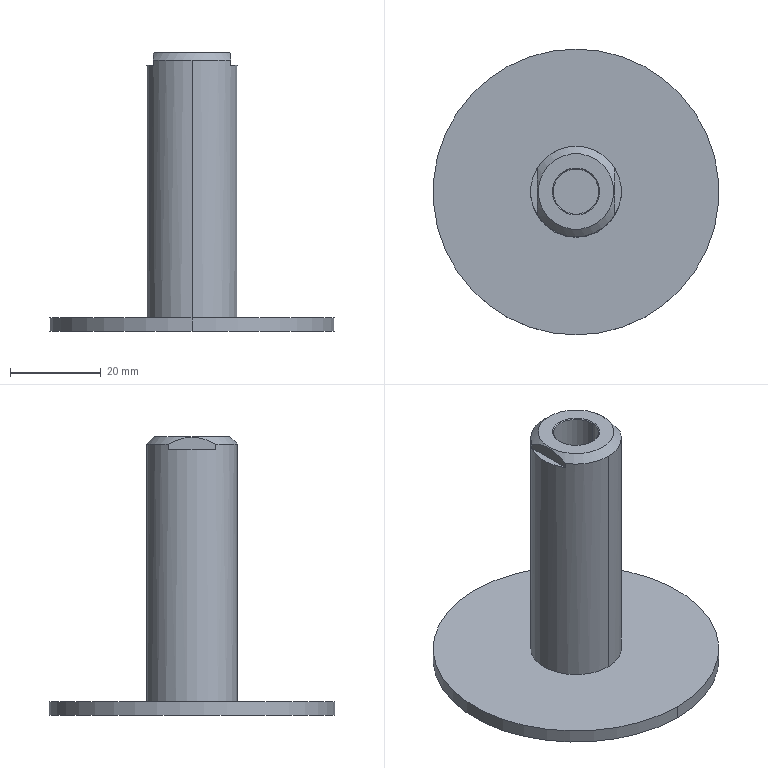Part | SolidWorks | features BaseBody 1 | 1 solid | 18 faces | box 63 x 63 x 61.5 mm | volume 26825 mm3 | plane 8 | cylinder 6 | cone 4 | commonest cylinder face diameters 10 x2 20 x2 63 x2
STEP:
#1=CARTESIAN_POINT('',(0.,-31.5,-49.667));
#2=VERTEX_POINT('',#1);
#3=CARTESIAN_POINT('',(0.,31.5,-49.667));
#4=VERTEX_POINT('',#3);
#5=CARTESIAN_POINT('',(0.,0.,-49.667));
#6=DIRECTION('',(0.,0.,1.));
#7=DIRECTION('',(0.,-1.,0.));
#8=AXIS2_PLACEMENT_3D('',#5,#6,#7);
#9=CIRCLE('',#8,31.5);
#10=EDGE_CURVE('',#2,#4,#9,.T.);
#11=ORIENTED_EDGE('',*,*,#10,.T.);
#12=CARTESIAN_POINT('',(0.,31.5,-46.667));
#13=VERTEX_POINT('',#12);
#14=CARTESIAN_POINT('',(0.,31.5,2.833));
#15=DIRECTION('',(0.,0.,1.));
#16=VECTOR('',#15,1000.);
#17=LINE('',#14,#16);
#18=EDGE_CURVE('',#4,#13,#17,.T.);
#19=ORIENTED_EDGE('',*,*,#18,.T.);
#20=CARTESIAN_POINT('',(0.,-31.5,-46.667));
#21=VERTEX_POINT('',#20);
#22=CARTESIAN_POINT('',(0.,0.,-46.667));
#23=DIRECTION('',(0.,0.,-1.));
#24=DIRECTION('',(0.,-1.,0.));
#25=AXIS2_PLACEMENT_3D('',#22,#23,#24);
#26=CIRCLE('',#25,31.5);
#27=EDGE_CURVE('',#13,#21,#26,.T.);
#28=ORIENTED_EDGE('',*,*,#27,.T.);
#29=CARTESIAN_POINT('',(0.,-31.5,2.833));
#30=DIRECTION('',(0.,0.,1.));
#31=VECTOR('',#30,1000.);
#32=LINE('',#29,#31);
#33=EDGE_CURVE('',#2,#21,#32,.T.);
#34=ORIENTED_EDGE('',*,*,#33,.F.);
#35=EDGE_LOOP('',(#11,#19,#28,#34));
#36=FACE_OUTER_BOUND('',#35,.T.);
#37=CARTESIAN_POINT('',(0.,0.,2.833));
#38=DIRECTION('',(0.,0.,1.));
#39=DIRECTION('',(0.,-1.,0.));
#40=AXIS2_PLACEMENT_3D('',#37,#38,#39);
#41=CYLINDRICAL_SURFACE('',#40,31.5);
#42=ADVANCED_FACE('',(#36),#41,.T.);
#43=CARTESIAN_POINT('',(0.,-10.,-46.667));
#44=VERTEX_POINT('',#43);
#45=CARTESIAN_POINT('',(0.,10.,-46.667));
#46=VERTEX_POINT('',#45);
#47=CARTESIAN_POINT('',(0.,0.,-46.667));
#48=DIRECTION('',(0.,0.,1.));
#49=DIRECTION('',(0.,-1.,0.));
#50=AXIS2_PLACEMENT_3D('',#47,#48,#49);
#51=CIRCLE('',#50,10.);
#52=EDGE_CURVE('',#44,#46,#51,.T.);
#53=ORIENTED_EDGE('',*,*,#52,.T.);
#54=CARTESIAN_POINT('',(0.,10.,10.167));
#55=VERTEX_POINT('',#54);
#56=CARTESIAN_POINT('',(0.,10.,2.833));
#57=DIRECTION('',(0.,0.,1.));
#58=VECTOR('',#57,1000.);
#59=LINE('',#56,#58);
#60=EDGE_CURVE('',#46,#55,#59,.T.);
#61=ORIENTED_EDGE('',*,*,#60,.T.);
#62=CARTESIAN_POINT('',(8.5,5.268,10.167));
#63=VERTEX_POINT('',#62);
#64=CARTESIAN_POINT('',(0.,0.,10.167));
#65=DIRECTION('',(0.,0.,-1.));
#66=DIRECTION('',(0.,-1.,0.));
#67=AXIS2_PLACEMENT_3D('',#64,#65,#66);
#68=CIRCLE('',#67,10.);
#69=EDGE_CURVE('',#55,#63,#68,.T.);
#70=ORIENTED_EDGE('',*,*,#69,.T.);
#71=CARTESIAN_POINT('',(8.5,5.268,9.033));
#72=VERTEX_POINT('',#71);
#73=CARTESIAN_POINT('',(8.5,5.268,9.033));
#74=DIRECTION('',(0.,0.,-1.));
#75=VECTOR('',#74,1000.);
#76=LINE('',#73,#75);
#77=EDGE_CURVE('',#63,#72,#76,.T.);
#78=ORIENTED_EDGE('',*,*,#77,.T.);
#79=CARTESIAN_POINT('',(8.5,-5.268,9.033));
#80=VERTEX_POINT('',#79);
#81=CARTESIAN_POINT('',(0.,0.,9.033));
#82=DIRECTION('',(0.,0.,-1.));
#83=DIRECTION('',(0.,-1.,0.));
#84=AXIS2_PLACEMENT_3D('',#81,#82,#83);
#85=CIRCLE('',#84,10.);
#86=EDGE_CURVE('',#72,#80,#85,.T.);
#87=ORIENTED_EDGE('',*,*,#86,.T.);
#88=CARTESIAN_POINT('',(8.5,-5.268,10.167));
#89=VERTEX_POINT('',#88);
#90=CARTESIAN_POINT('',(8.5,-5.268,9.033));
#91=DIRECTION('',(0.,0.,1.));
#92=VECTOR('',#91,1000.);
#93=LINE('',#90,#92);
#94=EDGE_CURVE('',#80,#89,#93,.T.);
#95=ORIENTED_EDGE('',*,*,#94,.T.);
#96=CARTESIAN_POINT('',(0.,-10.,10.167));
#97=VERTEX_POINT('',#96);
#98=CARTESIAN_POINT('',(0.,0.,10.167));
#99=DIRECTION('',(0.,0.,-1.));
#100=DIRECTION('',(0.,-1.,0.));
#101=AXIS2_PLACEMENT_3D('',#98,#99,#100);
#102=CIRCLE('',#101,10.);
#103=EDGE_CURVE('',#89,#97,#102,.T.);
#104=ORIENTED_EDGE('',*,*,#103,.T.);
#105=CARTESIAN_POINT('',(0.,-10.,2.833));
#106=DIRECTION('',(0.,0.,1.));
#107=VECTOR('',#106,1000.);
#108=LINE('',#105,#107);
#109=EDGE_CURVE('',#44,#97,#108,.T.);
#110=ORIENTED_EDGE('',*,*,#109,.F.);
#111=EDGE_LOOP('',(#53,#61,#70,#78,#87,#95,#104,#110));
#112=FACE_OUTER_BOUND('',#111,.T.);
#113=CARTESIAN_POINT('',(0.,0.,2.833));
#114=DIRECTION('',(0.,0.,1.));
#115=DIRECTION('',(0.,-1.,0.));
#116=AXIS2_PLACEMENT_3D('',#113,#114,#115);
#117=CYLINDRICAL_SURFACE('',#116,10.);
#118=ADVANCED_FACE('',(#112),#117,.T.);
#119=CARTESIAN_POINT('',(-8.333,0.,11.833));
#120=VERTEX_POINT('',#119);
#121=CARTESIAN_POINT('',(8.333,0.,11.833));
#122=VERTEX_POINT('',#121);
#123=CARTESIAN_POINT('',(0.,0.,11.833));
#124=DIRECTION('',(0.,0.,-1.));
#125=DIRECTION('',(-1.,0.,0.));
#126=AXIS2_PLACEMENT_3D('',#123,#124,#125);
#127=CIRCLE('',#126,8.333);
#128=EDGE_CURVE('',#120,#122,#127,.T.);
#129=ORIENTED_EDGE('',*,*,#128,.T.);
#130=CARTESIAN_POINT('',(8.5,0.,11.667));
#131=VERTEX_POINT('',#130);
#132=CARTESIAN_POINT('',(10.,0.,10.167));
#133=DIRECTION('',(0.7071,0.,-0.7071));
#134=VECTOR('',#133,1000.);
#135=LINE('',#132,#134);
#136=EDGE_CURVE('',#122,#131,#135,.T.);
#137=ORIENTED_EDGE('',*,*,#136,.T.);
#138=CARTESIAN_POINT('',(8.5,0.,11.667));
#139=CARTESIAN_POINT('',(8.5,0.459,11.667));
#140=CARTESIAN_POINT('',(8.5,0.9179,11.629));
#141=CARTESIAN_POINT('',(8.5,1.835,11.483));
#142=CARTESIAN_POINT('',(8.5,2.287,11.374));
#143=CARTESIAN_POINT('',(8.5,3.607,10.971));
#144=CARTESIAN_POINT('',(8.5,4.448,10.599));
#145=CARTESIAN_POINT('',(8.5,5.268,10.167));
#146=B_SPLINE_CURVE_WITH_KNOTS('',3,(#138,#139,#140,#141,#142,#143,#144,#145),.UNSPECIFIED.,.F.,.F.,(4,2,2,4),(0.005508,0.006884,0.008261,0.01101),.UNSPECIFIED.);
#147=EDGE_CURVE('',#131,#63,#146,.T.);
#148=ORIENTED_EDGE('',*,*,#147,.T.);
#149=ORIENTED_EDGE('',*,*,#69,.F.);
#150=CARTESIAN_POINT('',(-8.5,5.268,10.167));
#151=VERTEX_POINT('',#150);
#152=CARTESIAN_POINT('',(0.,0.,10.167));
#153=DIRECTION('',(0.,0.,-1.));
#154=DIRECTION('',(0.,-1.,0.));
#155=AXIS2_PLACEMENT_3D('',#152,#153,#154);
#156=CIRCLE('',#155,10.);
#157=EDGE_CURVE('',#151,#55,#156,.T.);
#158=ORIENTED_EDGE('',*,*,#157,.F.);
#159=CARTESIAN_POINT('',(-8.5,0.,11.667));
#160=VERTEX_POINT('',#159);
#161=CARTESIAN_POINT('',(-8.5,5.268,10.167));
#162=CARTESIAN_POINT('',(-8.5,4.448,10.599));
#163=CARTESIAN_POINT('',(-8.5,3.607,10.971));
#164=CARTESIAN_POINT('',(-8.5,2.288,11.374));
#165=CARTESIAN_POINT('',(-8.5,1.837,11.482));
#166=CARTESIAN_POINT('',(-8.5,0.9184,11.629));
#167=CARTESIAN_POINT('',(-8.5,0.4592,11.667));
#168=CARTESIAN_POINT('',(-8.5,0.,11.667));
#169=B_SPLINE_CURVE_WITH_KNOTS('',3,(#161,#162,#163,#164,#165,#166,#167,#168),.UNSPECIFIED.,.F.,.F.,(4,2,2,4),(0.,0.002754,0.004131,0.005508),.UNSPECIFIED.);
#170=EDGE_CURVE('',#151,#160,#169,.T.);
#171=ORIENTED_EDGE('',*,*,#170,.T.);
#172=CARTESIAN_POINT('',(-10.,0.,10.167));
#173=DIRECTION('',(-0.7071,0.,-0.7071));
#174=VECTOR('',#173,1000.);
#175=LINE('',#172,#174);
#176=EDGE_CURVE('',#120,#160,#175,.T.);
#177=ORIENTED_EDGE('',*,*,#176,.F.);
#178=EDGE_LOOP('',(#129,#137,#148,#149,#158,#171,#177));
#179=FACE_OUTER_BOUND('',#178,.T.);
#180=CARTESIAN_POINT('',(0.,0.,10.167));
#181=DIRECTION('',(0.,0.,-1.));
#182=DIRECTION('',(-1.,0.,0.));
#183=AXIS2_PLACEMENT_3D('',#180,#181,#182);
#184=CONICAL_SURFACE('',#183,10.,0.7854);
#185=ADVANCED_FACE('',(#179),#184,.T.);
#186=CARTESIAN_POINT('',(-5.,0.,11.633));
#187=VERTEX_POINT('',#186);
#188=CARTESIAN_POINT('',(5.,0.,11.633));
#189=VERTEX_POINT('',#188);
#190=CARTESIAN_POINT('',(0.,0.,11.633));
#191=DIRECTION('',(0.,0.,1.));
#192=DIRECTION('',(1.,0.,0.));
#193=AXIS2_PLACEMENT_3D('',#190,#191,#192);
#194=CIRCLE('',#193,5.);
#195=EDGE_CURVE('',#187,#189,#194,.T.);
#196=ORIENTED_EDGE('',*,*,#195,.F.);
#197=CARTESIAN_POINT('',(-5.2,0.,11.833));
#198=VERTEX_POINT('',#197);
#199=CARTESIAN_POINT('',(-5.2,0.,11.833));
#200=DIRECTION('',(-0.7071,0.,0.7071));
#201=VECTOR('',#200,1000.);
#202=LINE('',#199,#201);
#203=EDGE_CURVE('',#187,#198,#202,.T.);
#204=ORIENTED_EDGE('',*,*,#203,.T.);
#205=CARTESIAN_POINT('',(5.2,0.,11.833));
#206=VERTEX_POINT('',#205);
#207=CARTESIAN_POINT('',(0.,0.,11.833));
#208=DIRECTION('',(0.,0.,1.));
#209=DIRECTION('',(1.,0.,0.));
#210=AXIS2_PLACEMENT_3D('',#207,#208,#209);
#211=CIRCLE('',#210,5.2);
#212=EDGE_CURVE('',#198,#206,#211,.T.);
#213=ORIENTED_EDGE('',*,*,#212,.T.);
#214=CARTESIAN_POINT('',(5.2,0.,11.833));
#215=DIRECTION('',(0.7071,0.,0.7071));
#216=VECTOR('',#215,1000.);
#217=LINE('',#214,#216);
#218=EDGE_CURVE('',#189,#206,#217,.T.);
#219=ORIENTED_EDGE('',*,*,#218,.F.);
#220=EDGE_LOOP('',(#196,#204,#213,#219));
#221=FACE_OUTER_BOUND('',#220,.T.);
#222=CARTESIAN_POINT('',(0.,0.,11.833));
#223=DIRECTION('',(0.,0.,1.));
#224=DIRECTION('',(1.,0.,0.));
#225=AXIS2_PLACEMENT_3D('',#222,#223,#224);
#226=CONICAL_SURFACE('',#225,5.2,0.7854);
#227=ADVANCED_FACE('',(#221),#226,.F.);
#228=CARTESIAN_POINT('',(-5.,0.,1.833));
#229=VERTEX_POINT('',#228);
#230=CARTESIAN_POINT('',(5.,0.,1.833));
#231=VERTEX_POINT('',#230);
#232=CARTESIAN_POINT('',(0.,0.,1.833));
#233=DIRECTION('',(0.,0.,1.));
#234=DIRECTION('',(1.,0.,0.));
#235=AXIS2_PLACEMENT_3D('',#232,#233,#234);
#236=CIRCLE('',#235,5.);
#237=EDGE_CURVE('',#229,#231,#236,.T.);
#238=ORIENTED_EDGE('',*,*,#237,.F.);
#239=CARTESIAN_POINT('',(-5.,0.,1.833));
#240=DIRECTION('',(0.,0.,1.));
#241=VECTOR('',#240,1000.);
#242=LINE('',#239,#241);
#243=EDGE_CURVE('',#229,#187,#242,.T.);
#244=ORIENTED_EDGE('',*,*,#243,.T.);
#245=ORIENTED_EDGE('',*,*,#195,.T.);
#246=CARTESIAN_POINT('',(5.,0.,1.833));
#247=DIRECTION('',(0.,0.,1.));
#248=VECTOR('',#247,1000.);
#249=LINE('',#246,#248);
#250=EDGE_CURVE('',#231,#189,#249,.T.);
#251=ORIENTED_EDGE('',*,*,#250,.F.);
#252=EDGE_LOOP('',(#238,#244,#245,#251));
#253=FACE_OUTER_BOUND('',#252,.T.);
#254=CARTESIAN_POINT('',(0.,0.,1.833));
#255=DIRECTION('',(0.,0.,1.));
#256=DIRECTION('',(1.,0.,0.));
#257=AXIS2_PLACEMENT_3D('',#254,#255,#256);
#258=CYLINDRICAL_SURFACE('',#257,5.);
#259=ADVANCED_FACE('',(#253),#258,.F.);
#260=ORIENTED_EDGE('',*,*,#10,.F.);
#261=CARTESIAN_POINT('',(0.,0.,-49.667));
#262=DIRECTION('',(0.,0.,1.));
#263=DIRECTION('',(0.,-1.,0.));
#264=AXIS2_PLACEMENT_3D('',#261,#262,#263);
#265=CIRCLE('',#264,31.5);
#266=EDGE_CURVE('',#4,#2,#265,.T.);
#267=ORIENTED_EDGE('',*,*,#266,.F.);
#268=EDGE_LOOP('',(#260,#267));
#269=FACE_OUTER_BOUND('',#268,.T.);
#270=CARTESIAN_POINT('',(0.,31.5,-49.667));
#271=DIRECTION('',(0.,0.,1.));
#272=DIRECTION('',(0.,-1.,0.));
#273=AXIS2_PLACEMENT_3D('',#270,#271,#272);
#274=PLANE('',#273);
#275=ADVANCED_FACE('',(#269),#274,.F.);
#276=ORIENTED_EDGE('',*,*,#18,.F.);
#277=ORIENTED_EDGE('',*,*,#266,.T.);
#278=ORIENTED_EDGE('',*,*,#33,.T.);
#279=CARTESIAN_POINT('',(0.,0.,-46.667));
#280=DIRECTION('',(0.,0.,-1.));
#281=DIRECTION('',(0.,-1.,0.));
#282=AXIS2_PLACEMENT_3D('',#279,#280,#281);
#283=CIRCLE('',#282,31.5);
#284=EDGE_CURVE('',#21,#13,#283,.T.);
#285=ORIENTED_EDGE('',*,*,#284,.T.);
#286=EDGE_LOOP('',(#276,#277,#278,#285));
#287=FACE_OUTER_BOUND('',#286,.T.);
#288=CARTESIAN_POINT('',(0.,0.,2.833));
#289=DIRECTION('',(0.,0.,1.));
#290=DIRECTION('',(0.,-1.,0.));
#291=AXIS2_PLACEMENT_3D('',#288,#289,#290);
#292=CYLINDRICAL_SURFACE('',#291,31.5);
#293=ADVANCED_FACE('',(#287),#292,.T.);
#294=ORIENTED_EDGE('',*,*,#284,.F.);
#295=ORIENTED_EDGE('',*,*,#27,.F.);
#296=EDGE_LOOP('',(#294,#295));
#297=FACE_OUTER_BOUND('',#296,.T.);
#298=ORIENTED_EDGE('',*,*,#52,.F.);
#299=CARTESIAN_POINT('',(0.,0.,-46.667));
#300=DIRECTION('',(0.,0.,1.));
#301=DIRECTION('',(0.,-1.,0.));
#302=AXIS2_PLACEMENT_3D('',#299,#300,#301);
#303=CIRCLE('',#302,10.);
#304=EDGE_CURVE('',#46,#44,#303,.T.);
#305=ORIENTED_EDGE('',*,*,#304,.F.);
#306=EDGE_LOOP('',(#298,#305));
#307=FACE_BOUND('',#306,.T.);
#308=CARTESIAN_POINT('',(0.,31.5,-46.667));
#309=DIRECTION('',(0.,0.,-1.));
#310=DIRECTION('',(0.,1.,0.));
#311=AXIS2_PLACEMENT_3D('',#308,#309,#310);
#312=PLANE('',#311);
#313=ADVANCED_FACE('',(#297,#307),#312,.F.);
#314=ORIENTED_EDGE('',*,*,#60,.F.);
#315=ORIENTED_EDGE('',*,*,#304,.T.);
#316=ORIENTED_EDGE('',*,*,#109,.T.);
#317=CARTESIAN_POINT('',(-8.5,-5.268,10.167));
#318=VERTEX_POINT('',#317);
#319=CARTESIAN_POINT('',(0.,0.,10.167));
#320=DIRECTION('',(0.,0.,-1.));
#321=DIRECTION('',(0.,-1.,0.));
#322=AXIS2_PLACEMENT_3D('',#319,#320,#321);
#323=CIRCLE('',#322,10.);
#324=EDGE_CURVE('',#97,#318,#323,.T.);
#325=ORIENTED_EDGE('',*,*,#324,.T.);
#326=CARTESIAN_POINT('',(-8.5,-5.268,9.033));
#327=VERTEX_POINT('',#326);
#328=CARTESIAN_POINT('',(-8.5,-5.268,9.033));
#329=DIRECTION('',(0.,0.,-1.));
#330=VECTOR('',#329,1000.);
#331=LINE('',#328,#330);
#332=EDGE_CURVE('',#318,#327,#331,.T.);
#333=ORIENTED_EDGE('',*,*,#332,.T.);
#334=CARTESIAN_POINT('',(-8.5,5.268,9.033));
#335=VERTEX_POINT('',#334);
#336=CARTESIAN_POINT('',(0.,0.,9.033));
#337=DIRECTION('',(0.,0.,-1.));
#338=DIRECTION('',(0.,-1.,0.));
#339=AXIS2_PLACEMENT_3D('',#336,#337,#338);
#340=CIRCLE('',#339,10.);
#341=EDGE_CURVE('',#327,#335,#340,.T.);
#342=ORIENTED_EDGE('',*,*,#341,.T.);
#343=CARTESIAN_POINT('',(-8.5,5.268,9.033));
#344=DIRECTION('',(0.,0.,1.));
#345=VECTOR('',#344,1000.);
#346=LINE('',#343,#345);
#347=EDGE_CURVE('',#335,#151,#346,.T.);
#348=ORIENTED_EDGE('',*,*,#347,.T.);
#349=ORIENTED_EDGE('',*,*,#157,.T.);
#350=EDGE_LOOP('',(#314,#315,#316,#325,#333,#342,#348,#349));
#351=FACE_OUTER_BOUND('',#350,.T.);
#352=CARTESIAN_POINT('',(0.,0.,2.833));
#353=DIRECTION('',(0.,0.,1.));
#354=DIRECTION('',(0.,-1.,0.));
#355=AXIS2_PLACEMENT_3D('',#352,#353,#354);
#356=CYLINDRICAL_SURFACE('',#355,10.);
#357=ADVANCED_FACE('',(#351),#356,.T.);
#358=ORIENTED_EDGE('',*,*,#136,.F.);
#359=CARTESIAN_POINT('',(0.,0.,11.833));
#360=DIRECTION('',(0.,0.,-1.));
#361=DIRECTION('',(-1.,0.,0.));
#362=AXIS2_PLACEMENT_3D('',#359,#360,#361);
#363=CIRCLE('',#362,8.333);
#364=EDGE_CURVE('',#122,#120,#363,.T.);
#365=ORIENTED_EDGE('',*,*,#364,.T.);
#366=ORIENTED_EDGE('',*,*,#176,.T.);
#367=CARTESIAN_POINT('',(-8.5,0.,11.667));
#368=CARTESIAN_POINT('',(-8.5,-0.459,11.667));
#369=CARTESIAN_POINT('',(-8.5,-0.9179,11.629));
#370=CARTESIAN_POINT('',(-8.5,-1.835,11.483));
#371=CARTESIAN_POINT('',(-8.5,-2.287,11.374));
#372=CARTESIAN_POINT('',(-8.5,-3.607,10.971));
#373=CARTESIAN_POINT('',(-8.5,-4.448,10.599));
#374=CARTESIAN_POINT('',(-8.5,-5.268,10.167));
#375=B_SPLINE_CURVE_WITH_KNOTS('',3,(#367,#368,#369,#370,#371,#372,#373,#374),.UNSPECIFIED.,.F.,.F.,(4,2,2,4),(0.005508,0.006884,0.008261,0.01101),.UNSPECIFIED.);
#376=EDGE_CURVE('',#160,#318,#375,.T.);
#377=ORIENTED_EDGE('',*,*,#376,.T.);
#378=ORIENTED_EDGE('',*,*,#324,.F.);
#379=ORIENTED_EDGE('',*,*,#103,.F.);
#380=CARTESIAN_POINT('',(8.5,-5.268,10.167));
#381=CARTESIAN_POINT('',(8.5,-4.448,10.599));
#382=CARTESIAN_POINT('',(8.5,-3.607,10.971));
#383=CARTESIAN_POINT('',(8.5,-2.288,11.374));
#384=CARTESIAN_POINT('',(8.5,-1.837,11.482));
#385=CARTESIAN_POINT('',(8.5,-0.9184,11.629));
#386=CARTESIAN_POINT('',(8.5,-0.4592,11.667));
#387=CARTESIAN_POINT('',(8.5,0.,11.667));
#388=B_SPLINE_CURVE_WITH_KNOTS('',3,(#380,#381,#382,#383,#384,#385,#386,#387),.UNSPECIFIED.,.F.,.F.,(4,2,2,4),(0.,0.002754,0.004131,0.005508),.UNSPECIFIED.);
#389=EDGE_CURVE('',#89,#131,#388,.T.);
#390=ORIENTED_EDGE('',*,*,#389,.T.);
#391=EDGE_LOOP('',(#358,#365,#366,#377,#378,#379,#390));
#392=FACE_OUTER_BOUND('',#391,.T.);
#393=CARTESIAN_POINT('',(0.,0.,10.167));
#394=DIRECTION('',(0.,0.,-1.));
#395=DIRECTION('',(-1.,0.,0.));
#396=AXIS2_PLACEMENT_3D('',#393,#394,#395);
#397=CONICAL_SURFACE('',#396,10.,0.7854);
#398=ADVANCED_FACE('',(#392),#397,.T.);
#399=ORIENTED_EDGE('',*,*,#86,.F.);
#400=CARTESIAN_POINT('',(8.5,11.,9.033));
#401=DIRECTION('',(0.,-1.,0.));
#402=VECTOR('',#401,1000.);
#403=LINE('',#400,#402);
#404=EDGE_CURVE('',#72,#80,#403,.T.);
#405=ORIENTED_EDGE('',*,*,#404,.T.);
#406=EDGE_LOOP('',(#399,#405));
#407=FACE_OUTER_BOUND('',#406,.T.);
#408=CARTESIAN_POINT('',(8.5,11.,9.033));
#409=DIRECTION('',(0.,0.,1.));
#410=DIRECTION('',(1.,0.,0.));
#411=AXIS2_PLACEMENT_3D('',#408,#409,#410);
#412=PLANE('',#411);
#413=ADVANCED_FACE('',(#407),#412,.T.);
#414=ORIENTED_EDGE('',*,*,#341,.F.);
#415=CARTESIAN_POINT('',(-8.5,-11.,9.033));
#416=DIRECTION('',(0.,-1.,0.));
#417=VECTOR('',#416,1000.);
#418=LINE('',#415,#417);
#419=EDGE_CURVE('',#335,#327,#418,.T.);
#420=ORIENTED_EDGE('',*,*,#419,.F.);
#421=EDGE_LOOP('',(#414,#420));
#422=FACE_OUTER_BOUND('',#421,.T.);
#423=CARTESIAN_POINT('',(-8.5,-11.,9.033));
#424=DIRECTION('',(0.,0.,-1.));
#425=DIRECTION('',(-1.,0.,0.));
#426=AXIS2_PLACEMENT_3D('',#423,#424,#425);
#427=PLANE('',#426);
#428=ADVANCED_FACE('',(#422),#427,.F.);
#429=ORIENTED_EDGE('',*,*,#77,.F.);
#430=ORIENTED_EDGE('',*,*,#147,.F.);
#431=ORIENTED_EDGE('',*,*,#389,.F.);
#432=ORIENTED_EDGE('',*,*,#94,.F.);
#433=ORIENTED_EDGE('',*,*,#404,.F.);
#434=EDGE_LOOP('',(#429,#430,#431,#432,#433));
#435=FACE_OUTER_BOUND('',#434,.T.);
#436=CARTESIAN_POINT('',(8.5,11.,9.033));
#437=DIRECTION('',(-1.,0.,0.));
#438=DIRECTION('',(0.,0.,1.));
#439=AXIS2_PLACEMENT_3D('',#436,#437,#438);
#440=PLANE('',#439);
#441=ADVANCED_FACE('',(#435),#440,.F.);
#442=ORIENTED_EDGE('',*,*,#128,.F.);
#443=ORIENTED_EDGE('',*,*,#364,.F.);
#444=EDGE_LOOP('',(#442,#443));
#445=FACE_OUTER_BOUND('',#444,.T.);
#446=CARTESIAN_POINT('',(0.,0.,11.833));
#447=DIRECTION('',(0.,0.,1.));
#448=DIRECTION('',(1.,0.,0.));
#449=AXIS2_PLACEMENT_3D('',#446,#447,#448);
#450=CIRCLE('',#449,5.2);
#451=EDGE_CURVE('',#206,#198,#450,.T.);
#452=ORIENTED_EDGE('',*,*,#451,.F.);
#453=ORIENTED_EDGE('',*,*,#212,.F.);
#454=EDGE_LOOP('',(#452,#453));
#455=FACE_BOUND('',#454,.T.);
#456=CARTESIAN_POINT('',(0.,0.,11.833));
#457=DIRECTION('',(0.,0.,-1.));
#458=DIRECTION('',(0.,1.,0.));
#459=AXIS2_PLACEMENT_3D('',#456,#457,#458);
#460=PLANE('',#459);
#461=ADVANCED_FACE('',(#445,#455),#460,.F.);
#462=ORIENTED_EDGE('',*,*,#332,.F.);
#463=ORIENTED_EDGE('',*,*,#376,.F.);
#464=ORIENTED_EDGE('',*,*,#170,.F.);
#465=ORIENTED_EDGE('',*,*,#347,.F.);
#466=ORIENTED_EDGE('',*,*,#419,.T.);
#467=EDGE_LOOP('',(#462,#463,#464,#465,#466));
#468=FACE_OUTER_BOUND('',#467,.T.);
#469=CARTESIAN_POINT('',(-8.5,11.,9.033));
#470=DIRECTION('',(1.,0.,0.));
#471=DIRECTION('',(0.,1.,0.));
#472=AXIS2_PLACEMENT_3D('',#469,#470,#471);
#473=PLANE('',#472);
#474=ADVANCED_FACE('',(#468),#473,.F.);
#475=ORIENTED_EDGE('',*,*,#203,.F.);
#476=CARTESIAN_POINT('',(0.,0.,11.633));
#477=DIRECTION('',(0.,0.,1.));
#478=DIRECTION('',(1.,0.,0.));
#479=AXIS2_PLACEMENT_3D('',#476,#477,#478);
#480=CIRCLE('',#479,5.);
#481=EDGE_CURVE('',#189,#187,#480,.T.);
#482=ORIENTED_EDGE('',*,*,#481,.F.);
#483=ORIENTED_EDGE('',*,*,#218,.T.);
#484=ORIENTED_EDGE('',*,*,#451,.T.);
#485=EDGE_LOOP('',(#475,#482,#483,#484));
#486=FACE_OUTER_BOUND('',#485,.T.);
#487=CARTESIAN_POINT('',(0.,0.,11.833));
#488=DIRECTION('',(0.,0.,1.));
#489=DIRECTION('',(1.,0.,0.));
#490=AXIS2_PLACEMENT_3D('',#487,#488,#489);
#491=CONICAL_SURFACE('',#490,5.2,0.7854);
#492=ADVANCED_FACE('',(#486),#491,.F.);
#493=ORIENTED_EDGE('',*,*,#243,.F.);
#494=CARTESIAN_POINT('',(0.,0.,1.833));
#495=DIRECTION('',(0.,0.,1.));
#496=DIRECTION('',(1.,0.,0.));
#497=AXIS2_PLACEMENT_3D('',#494,#495,#496);
#498=CIRCLE('',#497,5.);
#499=EDGE_CURVE('',#231,#229,#498,.T.);
#500=ORIENTED_EDGE('',*,*,#499,.F.);
#501=ORIENTED_EDGE('',*,*,#250,.T.);
#502=ORIENTED_EDGE('',*,*,#481,.T.);
#503=EDGE_LOOP('',(#493,#500,#501,#502));
#504=FACE_OUTER_BOUND('',#503,.T.);
#505=CARTESIAN_POINT('',(0.,0.,1.833));
#506=DIRECTION('',(0.,0.,1.));
#507=DIRECTION('',(1.,0.,0.));
#508=AXIS2_PLACEMENT_3D('',#505,#506,#507);
#509=CYLINDRICAL_SURFACE('',#508,5.);
#510=ADVANCED_FACE('',(#504),#509,.F.);
#511=ORIENTED_EDGE('',*,*,#499,.T.);
#512=ORIENTED_EDGE('',*,*,#237,.T.);
#513=EDGE_LOOP('',(#511,#512));
#514=FACE_OUTER_BOUND('',#513,.T.);
#515=CARTESIAN_POINT('',(0.,0.,1.833));
#516=DIRECTION('',(0.,0.,1.));
#517=DIRECTION('',(1.,0.,0.));
#518=AXIS2_PLACEMENT_3D('',#515,#516,#517);
#519=PLANE('',#518);
#520=ADVANCED_FACE('',(#514),#519,.T.);
#521=CLOSED_SHELL('',(#42,#118,#185,#227,#259,#275,#293,#313,#357,#398,#413,#428,#441,#461,#474,#492,#510,#520));
#522=MANIFOLD_SOLID_BREP('',#521);
#523=CARTESIAN_POINT('',(0.,0.,0.));
#524=DIRECTION('',(0.,0.,1.));
#525=DIRECTION('',(1.,0.,0.));
#526=AXIS2_PLACEMENT_3D('',#523,#524,#525);
#527=(LENGTH_UNIT()NAMED_UNIT(*)SI_UNIT(.MILLI.,.METRE.));
#528=UNCERTAINTY_MEASURE_WITH_UNIT(LENGTH_MEASURE(0.00001),#527,'','');
#529=(NAMED_UNIT(*)PLANE_ANGLE_UNIT()SI_UNIT($,.RADIAN.));
#530=(NAMED_UNIT(*)SI_UNIT($,.STERADIAN.)SOLID_ANGLE_UNIT());
#531=(GEOMETRIC_REPRESENTATION_CONTEXT(3)GLOBAL_UNCERTAINTY_ASSIGNED_CONTEXT((#528))GLOBAL_UNIT_ASSIGNED_CONTEXT((#527,#529,#530))REPRESENTATION_CONTEXT('',''));
#532=ADVANCED_BREP_SHAPE_REPRESENTATION('',(#522,#526),#531);